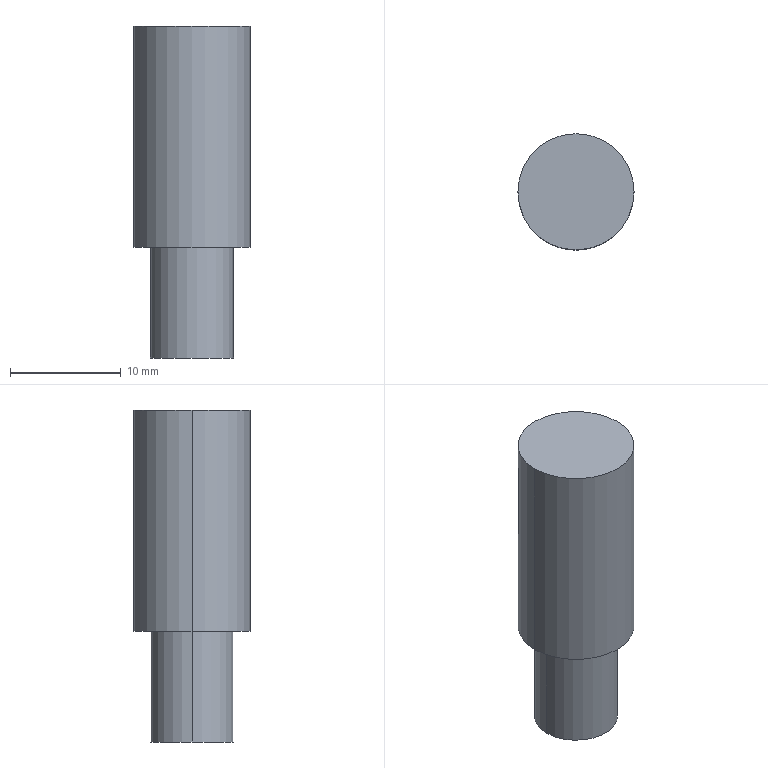Part | Creo | features DATUM PLANE 3, CURVE 2, PROTRUSION 2, COORDINATE SYSTEM 1 | 1 solid | 7 faces | box 10.5 x 10.5 x 30 mm | volume 2174 mm3 | cylinder 4 | plane 3 | commonest cylinder face diameters 7.5 x2 10.5 x2
STEP:
#1=CARTESIAN_POINT('',(0.,0.,0.));
#2=DIRECTION('',(0.,0.,1.));
#3=DIRECTION('',(1.,0.,0.));
#4=AXIS2_PLACEMENT_3D('',#1,#2,#3);
#5=CARTESIAN_POINT('',(3.75,0.,0.));
#6=VERTEX_POINT('',#5);
#7=CARTESIAN_POINT('',(-3.75,0.,0.));
#8=VERTEX_POINT('',#7);
#9=CARTESIAN_POINT('',(0.,0.,0.));
#10=DIRECTION('',(0.,0.,1.));
#11=DIRECTION('',(1.,0.,0.));
#12=AXIS2_PLACEMENT_3D('',#9,#10,#11);
#13=CIRCLE('',#12,3.75);
#14=EDGE_CURVE('',#6,#8,#13,.T.);
#15=ORIENTED_EDGE('',*,*,#14,.T.);
#16=CARTESIAN_POINT('',(0.,0.,0.));
#17=DIRECTION('',(0.,0.,1.));
#18=DIRECTION('',(-1.,0.,0.));
#19=AXIS2_PLACEMENT_3D('',#16,#17,#18);
#20=CIRCLE('',#19,3.75);
#21=EDGE_CURVE('',#8,#6,#20,.T.);
#22=ORIENTED_EDGE('',*,*,#21,.T.);
#23=EDGE_LOOP('',(#15,#22));
#24=FACE_OUTER_BOUND('',#23,.F.);
#25=CARTESIAN_POINT('',(0.,0.,0.));
#26=DIRECTION('',(0.,0.,1.));
#27=DIRECTION('',(1.,0.,0.));
#28=AXIS2_PLACEMENT_3D('',#25,#26,#27);
#29=PLANE('',#28);
#30=ADVANCED_FACE('',(#24),#29,.F.);
#31=CARTESIAN_POINT('',(3.75,0.,10.));
#32=VERTEX_POINT('',#31);
#33=CARTESIAN_POINT('',(-3.75,0.,10.));
#34=VERTEX_POINT('',#33);
#35=CARTESIAN_POINT('',(0.,0.,10.));
#36=DIRECTION('',(0.,0.,1.));
#37=DIRECTION('',(1.,0.,0.));
#38=AXIS2_PLACEMENT_3D('',#35,#36,#37);
#39=CIRCLE('',#38,3.75);
#40=EDGE_CURVE('',#32,#34,#39,.T.);
#41=ORIENTED_EDGE('',*,*,#40,.T.);
#42=CARTESIAN_POINT('',(-3.75,0.,0.));
#43=DIRECTION('',(0.,0.,1.));
#44=VECTOR('',#43,10.);
#45=LINE('',#42,#44);
#46=EDGE_CURVE('',#8,#34,#45,.T.);
#47=ORIENTED_EDGE('',*,*,#46,.F.);
#48=ORIENTED_EDGE('',*,*,#14,.F.);
#49=CARTESIAN_POINT('',(3.75,0.,0.));
#50=DIRECTION('',(0.,0.,1.));
#51=VECTOR('',#50,10.);
#52=LINE('',#49,#51);
#53=EDGE_CURVE('',#6,#32,#52,.T.);
#54=ORIENTED_EDGE('',*,*,#53,.T.);
#55=EDGE_LOOP('',(#41,#47,#48,#54));
#56=FACE_OUTER_BOUND('',#55,.F.);
#57=CARTESIAN_POINT('',(0.,0.,0.));
#58=DIRECTION('',(0.,0.,1.));
#59=DIRECTION('',(1.,0.,0.));
#60=AXIS2_PLACEMENT_3D('',#57,#58,#59);
#61=CYLINDRICAL_SURFACE('',#60,3.75);
#62=ADVANCED_FACE('',(#56),#61,.T.);
#63=CARTESIAN_POINT('',(5.25,0.,10.));
#64=VERTEX_POINT('',#63);
#65=CARTESIAN_POINT('',(-5.25,0.,10.));
#66=VERTEX_POINT('',#65);
#67=CARTESIAN_POINT('',(0.,0.,10.));
#68=DIRECTION('',(0.,0.,1.));
#69=DIRECTION('',(1.,0.,0.));
#70=AXIS2_PLACEMENT_3D('',#67,#68,#69);
#71=CIRCLE('',#70,5.25);
#72=EDGE_CURVE('',#64,#66,#71,.T.);
#73=ORIENTED_EDGE('',*,*,#72,.T.);
#74=CARTESIAN_POINT('',(0.,0.,10.));
#75=DIRECTION('',(0.,0.,1.));
#76=DIRECTION('',(-1.,0.,0.));
#77=AXIS2_PLACEMENT_3D('',#74,#75,#76);
#78=CIRCLE('',#77,5.25);
#79=EDGE_CURVE('',#66,#64,#78,.T.);
#80=ORIENTED_EDGE('',*,*,#79,.T.);
#81=EDGE_LOOP('',(#73,#80));
#82=FACE_OUTER_BOUND('',#81,.F.);
#83=ORIENTED_EDGE('',*,*,#40,.F.);
#84=CARTESIAN_POINT('',(0.,0.,10.));
#85=DIRECTION('',(0.,0.,1.));
#86=DIRECTION('',(-1.,0.,0.));
#87=AXIS2_PLACEMENT_3D('',#84,#85,#86);
#88=CIRCLE('',#87,3.75);
#89=EDGE_CURVE('',#34,#32,#88,.T.);
#90=ORIENTED_EDGE('',*,*,#89,.F.);
#91=EDGE_LOOP('',(#83,#90));
#92=FACE_BOUND('',#91,.F.);
#93=CARTESIAN_POINT('',(0.,0.,10.));
#94=DIRECTION('',(0.,0.,1.));
#95=DIRECTION('',(1.,0.,0.));
#96=AXIS2_PLACEMENT_3D('',#93,#94,#95);
#97=PLANE('',#96);
#98=ADVANCED_FACE('',(#82,#92),#97,.F.);
#99=ORIENTED_EDGE('',*,*,#72,.F.);
#100=CARTESIAN_POINT('',(5.25,0.,30.));
#101=VERTEX_POINT('',#100);
#102=CARTESIAN_POINT('',(5.25,0.,10.));
#103=DIRECTION('',(0.,0.,1.));
#104=VECTOR('',#103,20.);
#105=LINE('',#102,#104);
#106=EDGE_CURVE('',#64,#101,#105,.T.);
#107=ORIENTED_EDGE('',*,*,#106,.T.);
#108=CARTESIAN_POINT('',(-5.25,0.,30.));
#109=VERTEX_POINT('',#108);
#110=CARTESIAN_POINT('',(0.,0.,30.));
#111=DIRECTION('',(0.,0.,1.));
#112=DIRECTION('',(1.,0.,0.));
#113=AXIS2_PLACEMENT_3D('',#110,#111,#112);
#114=CIRCLE('',#113,5.25);
#115=EDGE_CURVE('',#101,#109,#114,.T.);
#116=ORIENTED_EDGE('',*,*,#115,.T.);
#117=CARTESIAN_POINT('',(-5.25,0.,10.));
#118=DIRECTION('',(0.,0.,1.));
#119=VECTOR('',#118,20.);
#120=LINE('',#117,#119);
#121=EDGE_CURVE('',#66,#109,#120,.T.);
#122=ORIENTED_EDGE('',*,*,#121,.F.);
#123=EDGE_LOOP('',(#99,#107,#116,#122));
#124=FACE_OUTER_BOUND('',#123,.F.);
#125=CARTESIAN_POINT('',(0.,0.,10.));
#126=DIRECTION('',(0.,0.,1.));
#127=DIRECTION('',(1.,0.,0.));
#128=AXIS2_PLACEMENT_3D('',#125,#126,#127);
#129=CYLINDRICAL_SURFACE('',#128,5.25);
#130=ADVANCED_FACE('',(#124),#129,.T.);
#131=ORIENTED_EDGE('',*,*,#79,.F.);
#132=ORIENTED_EDGE('',*,*,#121,.T.);
#133=CARTESIAN_POINT('',(0.,0.,30.));
#134=DIRECTION('',(0.,0.,1.));
#135=DIRECTION('',(-1.,0.,0.));
#136=AXIS2_PLACEMENT_3D('',#133,#134,#135);
#137=CIRCLE('',#136,5.25);
#138=EDGE_CURVE('',#109,#101,#137,.T.);
#139=ORIENTED_EDGE('',*,*,#138,.T.);
#140=ORIENTED_EDGE('',*,*,#106,.F.);
#141=EDGE_LOOP('',(#131,#132,#139,#140));
#142=FACE_OUTER_BOUND('',#141,.F.);
#143=CARTESIAN_POINT('',(0.,0.,10.));
#144=DIRECTION('',(0.,0.,1.));
#145=DIRECTION('',(1.,0.,0.));
#146=AXIS2_PLACEMENT_3D('',#143,#144,#145);
#147=CYLINDRICAL_SURFACE('',#146,5.25);
#148=ADVANCED_FACE('',(#142),#147,.T.);
#149=ORIENTED_EDGE('',*,*,#115,.F.);
#150=ORIENTED_EDGE('',*,*,#138,.F.);
#151=EDGE_LOOP('',(#149,#150));
#152=FACE_OUTER_BOUND('',#151,.F.);
#153=CARTESIAN_POINT('',(0.,0.,30.));
#154=DIRECTION('',(0.,0.,1.));
#155=DIRECTION('',(1.,0.,0.));
#156=AXIS2_PLACEMENT_3D('',#153,#154,#155);
#157=PLANE('',#156);
#158=ADVANCED_FACE('',(#152),#157,.T.);
#159=ORIENTED_EDGE('',*,*,#89,.T.);
#160=ORIENTED_EDGE('',*,*,#53,.F.);
#161=ORIENTED_EDGE('',*,*,#21,.F.);
#162=ORIENTED_EDGE('',*,*,#46,.T.);
#163=EDGE_LOOP('',(#159,#160,#161,#162));
#164=FACE_OUTER_BOUND('',#163,.F.);
#165=CARTESIAN_POINT('',(0.,0.,0.));
#166=DIRECTION('',(0.,0.,1.));
#167=DIRECTION('',(1.,0.,0.));
#168=AXIS2_PLACEMENT_3D('',#165,#166,#167);
#169=CYLINDRICAL_SURFACE('',#168,3.75);
#170=ADVANCED_FACE('',(#164),#169,.T.);
#171=CLOSED_SHELL('',(#30,#62,#98,#130,#148,#158,#170));
#172=MANIFOLD_SOLID_BREP('',#171);
#173=(LENGTH_UNIT()NAMED_UNIT(*)SI_UNIT(.MILLI.,.METRE.));
#174=UNCERTAINTY_MEASURE_WITH_UNIT(LENGTH_MEASURE(0.003348),#173,'','');
#175=(NAMED_UNIT(*)PLANE_ANGLE_UNIT()SI_UNIT($,.RADIAN.));
#176=PLANE_ANGLE_MEASURE_WITH_UNIT(PLANE_ANGLE_MEASURE(0.01745),#175);
#177=(CONVERSION_BASED_UNIT('DEGREE',#176)NAMED_UNIT(*)PLANE_ANGLE_UNIT());
#178=(NAMED_UNIT(*)SI_UNIT($,.STERADIAN.)SOLID_ANGLE_UNIT());
#179=(GEOMETRIC_REPRESENTATION_CONTEXT(3)GLOBAL_UNCERTAINTY_ASSIGNED_CONTEXT((#174))GLOBAL_UNIT_ASSIGNED_CONTEXT((#173,#177,#178))REPRESENTATION_CONTEXT('',''));
#180=ADVANCED_BREP_SHAPE_REPRESENTATION('',(#4,#172),#179);